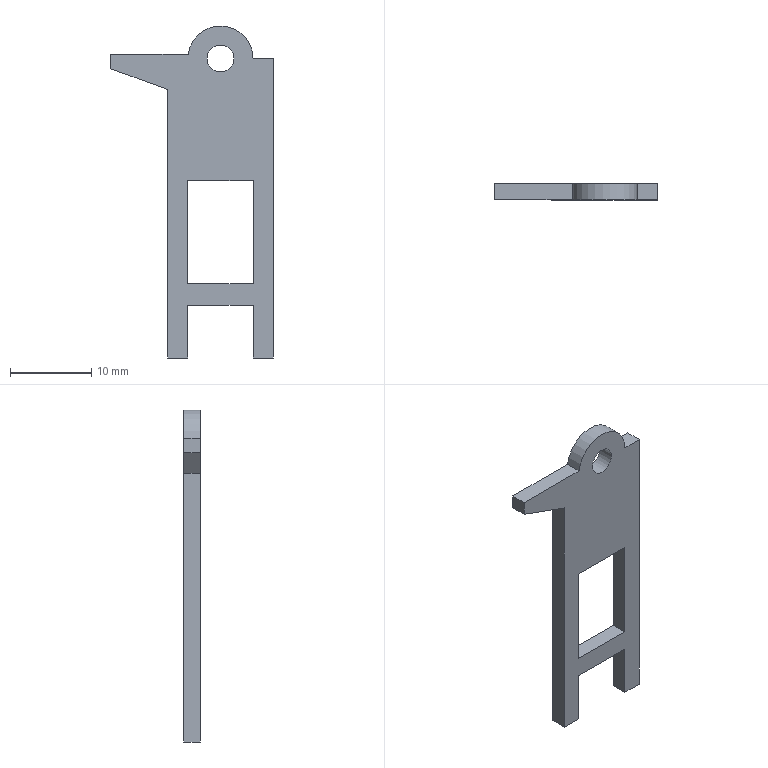Part | NX | 1 solid | 19 faces | box 20 x 2 x 40.8 mm | volume 727.635 mm3 | plane 17 | cylinder 2 | commonest cylinder face diameters 3.3 x1 8 x1
STEP:
#1=CARTESIAN_POINT('',(11.,81.5,41.85));
#2=VERTEX_POINT('',#1);
#3=CARTESIAN_POINT('',(11.,81.5,40.2));
#4=DIRECTION('',(0.,-1.,0.));
#5=DIRECTION('',(0.,0.,1.));
#6=AXIS2_PLACEMENT_3D('',#3,#4,#5);
#7=CIRCLE('',#6,1.65);
#8=EDGE_CURVE('',#2,#2,#7,.T.);
#9=ORIENTED_EDGE('',*,*,#8,.T.);
#10=EDGE_LOOP('',(#9));
#11=FACE_BOUND('',#10,.T.);
#12=CARTESIAN_POINT('',(4.5,81.5,3.4));
#13=VERTEX_POINT('',#12);
#14=CARTESIAN_POINT('',(7.,81.5,3.4));
#15=VERTEX_POINT('',#14);
#16=CARTESIAN_POINT('',(4.5,81.5,3.4));
#17=DIRECTION('',(1.,0.,0.));
#18=VECTOR('',#17,1000.);
#19=LINE('',#16,#18);
#20=EDGE_CURVE('',#13,#15,#19,.T.);
#21=ORIENTED_EDGE('',*,*,#20,.F.);
#22=CARTESIAN_POINT('',(4.5,81.5,36.4));
#23=VERTEX_POINT('',#22);
#24=CARTESIAN_POINT('',(4.5,81.5,3.4));
#25=DIRECTION('',(0.,0.,-1.));
#26=VECTOR('',#25,1000.);
#27=LINE('',#24,#26);
#28=EDGE_CURVE('',#23,#13,#27,.T.);
#29=ORIENTED_EDGE('',*,*,#28,.F.);
#30=CARTESIAN_POINT('',(-2.5,81.5,38.948));
#31=VERTEX_POINT('',#30);
#32=CARTESIAN_POINT('',(-2.5,81.5,38.948));
#33=DIRECTION('',(0.9397,0.,-0.342));
#34=VECTOR('',#33,1000.);
#35=LINE('',#32,#34);
#36=EDGE_CURVE('',#31,#23,#35,.T.);
#37=ORIENTED_EDGE('',*,*,#36,.F.);
#38=CARTESIAN_POINT('',(-2.5,81.5,40.7));
#39=VERTEX_POINT('',#38);
#40=CARTESIAN_POINT('',(-2.5,81.5,40.7));
#41=DIRECTION('',(0.,0.,-1.));
#42=VECTOR('',#41,1000.);
#43=LINE('',#40,#42);
#44=EDGE_CURVE('',#39,#31,#43,.T.);
#45=ORIENTED_EDGE('',*,*,#44,.F.);
#46=CARTESIAN_POINT('',(7.031,81.5,40.7));
#47=VERTEX_POINT('',#46);
#48=CARTESIAN_POINT('',(-2.5,81.5,40.7));
#49=DIRECTION('',(-1.,0.,0.));
#50=VECTOR('',#49,1000.);
#51=LINE('',#48,#50);
#52=EDGE_CURVE('',#47,#39,#51,.T.);
#53=ORIENTED_EDGE('',*,*,#52,.F.);
#54=CARTESIAN_POINT('',(15.,81.5,40.2));
#55=VERTEX_POINT('',#54);
#56=CARTESIAN_POINT('',(11.,81.5,40.2));
#57=DIRECTION('',(0.,-1.,0.));
#58=DIRECTION('',(0.,0.,-1.));
#59=AXIS2_PLACEMENT_3D('',#56,#57,#58);
#60=CIRCLE('',#59,4.);
#61=EDGE_CURVE('',#55,#47,#60,.T.);
#62=ORIENTED_EDGE('',*,*,#61,.F.);
#63=CARTESIAN_POINT('',(17.5,81.5,40.2));
#64=VERTEX_POINT('',#63);
#65=CARTESIAN_POINT('',(15.,81.5,40.2));
#66=DIRECTION('',(-1.,0.,0.));
#67=VECTOR('',#66,1000.);
#68=LINE('',#65,#67);
#69=EDGE_CURVE('',#64,#55,#68,.T.);
#70=ORIENTED_EDGE('',*,*,#69,.F.);
#71=CARTESIAN_POINT('',(17.5,81.5,3.4));
#72=VERTEX_POINT('',#71);
#73=CARTESIAN_POINT('',(17.5,81.5,3.4));
#74=DIRECTION('',(0.,0.,1.));
#75=VECTOR('',#74,1000.);
#76=LINE('',#73,#75);
#77=EDGE_CURVE('',#72,#64,#76,.T.);
#78=ORIENTED_EDGE('',*,*,#77,.F.);
#79=CARTESIAN_POINT('',(15.,81.5,3.4));
#80=VERTEX_POINT('',#79);
#81=CARTESIAN_POINT('',(15.,81.5,3.4));
#82=DIRECTION('',(1.,0.,0.));
#83=VECTOR('',#82,1000.);
#84=LINE('',#81,#83);
#85=EDGE_CURVE('',#80,#72,#84,.T.);
#86=ORIENTED_EDGE('',*,*,#85,.F.);
#87=CARTESIAN_POINT('',(15.,81.5,9.9));
#88=VERTEX_POINT('',#87);
#89=CARTESIAN_POINT('',(15.,81.5,3.4));
#90=DIRECTION('',(0.,0.,-1.));
#91=VECTOR('',#90,1000.);
#92=LINE('',#89,#91);
#93=EDGE_CURVE('',#88,#80,#92,.T.);
#94=ORIENTED_EDGE('',*,*,#93,.F.);
#95=CARTESIAN_POINT('',(7.,81.5,9.9));
#96=VERTEX_POINT('',#95);
#97=CARTESIAN_POINT('',(7.,81.5,9.9));
#98=DIRECTION('',(1.,0.,0.));
#99=VECTOR('',#98,1000.);
#100=LINE('',#97,#99);
#101=EDGE_CURVE('',#96,#88,#100,.T.);
#102=ORIENTED_EDGE('',*,*,#101,.F.);
#103=CARTESIAN_POINT('',(7.,81.5,3.4));
#104=DIRECTION('',(0.,0.,1.));
#105=VECTOR('',#104,1000.);
#106=LINE('',#103,#105);
#107=EDGE_CURVE('',#15,#96,#106,.T.);
#108=ORIENTED_EDGE('',*,*,#107,.F.);
#109=EDGE_LOOP('',(#21,#29,#37,#45,#53,#62,#70,#78,#86,#94,#102,#108));
#110=FACE_BOUND('',#109,.T.);
#111=CARTESIAN_POINT('',(7.,81.5,25.2));
#112=VERTEX_POINT('',#111);
#113=CARTESIAN_POINT('',(7.,81.5,12.5));
#114=VERTEX_POINT('',#113);
#115=CARTESIAN_POINT('',(7.,81.5,12.5));
#116=DIRECTION('',(0.,0.,-1.));
#117=VECTOR('',#116,1000.);
#118=LINE('',#115,#117);
#119=EDGE_CURVE('',#112,#114,#118,.T.);
#120=ORIENTED_EDGE('',*,*,#119,.T.);
#121=CARTESIAN_POINT('',(15.,81.5,12.5));
#122=VERTEX_POINT('',#121);
#123=CARTESIAN_POINT('',(7.,81.5,12.5));
#124=DIRECTION('',(1.,0.,0.));
#125=VECTOR('',#124,1000.);
#126=LINE('',#123,#125);
#127=EDGE_CURVE('',#114,#122,#126,.T.);
#128=ORIENTED_EDGE('',*,*,#127,.T.);
#129=CARTESIAN_POINT('',(15.,81.5,25.2));
#130=VERTEX_POINT('',#129);
#131=CARTESIAN_POINT('',(15.,81.5,12.5));
#132=DIRECTION('',(0.,0.,1.));
#133=VECTOR('',#132,1000.);
#134=LINE('',#131,#133);
#135=EDGE_CURVE('',#122,#130,#134,.T.);
#136=ORIENTED_EDGE('',*,*,#135,.T.);
#137=CARTESIAN_POINT('',(7.,81.5,25.2));
#138=DIRECTION('',(-1.,0.,0.));
#139=VECTOR('',#138,1000.);
#140=LINE('',#137,#139);
#141=EDGE_CURVE('',#130,#112,#140,.T.);
#142=ORIENTED_EDGE('',*,*,#141,.T.);
#143=EDGE_LOOP('',(#120,#128,#136,#142));
#144=FACE_BOUND('',#143,.T.);
#145=CARTESIAN_POINT('',(11.,81.5,40.2));
#146=DIRECTION('',(0.,1.,0.));
#147=DIRECTION('',(0.,0.,-1.));
#148=AXIS2_PLACEMENT_3D('',#145,#146,#147);
#149=PLANE('',#148);
#150=ADVANCED_FACE('',(#11,#110,#144),#149,.T.);
#151=CARTESIAN_POINT('',(11.,79.5,41.85));
#152=VERTEX_POINT('',#151);
#153=CARTESIAN_POINT('',(11.,79.5,40.2));
#154=DIRECTION('',(0.,-1.,0.));
#155=DIRECTION('',(0.,0.,1.));
#156=AXIS2_PLACEMENT_3D('',#153,#154,#155);
#157=CIRCLE('',#156,1.65);
#158=EDGE_CURVE('',#152,#152,#157,.T.);
#159=ORIENTED_EDGE('',*,*,#158,.F.);
#160=EDGE_LOOP('',(#159));
#161=FACE_BOUND('',#160,.T.);
#162=CARTESIAN_POINT('',(4.5,79.5,3.4));
#163=VERTEX_POINT('',#162);
#164=CARTESIAN_POINT('',(7.,79.5,3.4));
#165=VERTEX_POINT('',#164);
#166=CARTESIAN_POINT('',(4.5,79.5,3.4));
#167=DIRECTION('',(1.,0.,0.));
#168=VECTOR('',#167,1000.);
#169=LINE('',#166,#168);
#170=EDGE_CURVE('',#163,#165,#169,.T.);
#171=ORIENTED_EDGE('',*,*,#170,.T.);
#172=CARTESIAN_POINT('',(7.,79.5,9.9));
#173=VERTEX_POINT('',#172);
#174=CARTESIAN_POINT('',(7.,79.5,3.4));
#175=DIRECTION('',(0.,0.,1.));
#176=VECTOR('',#175,1000.);
#177=LINE('',#174,#176);
#178=EDGE_CURVE('',#165,#173,#177,.T.);
#179=ORIENTED_EDGE('',*,*,#178,.T.);
#180=CARTESIAN_POINT('',(15.,79.5,9.9));
#181=VERTEX_POINT('',#180);
#182=CARTESIAN_POINT('',(7.,79.5,9.9));
#183=DIRECTION('',(1.,0.,0.));
#184=VECTOR('',#183,1000.);
#185=LINE('',#182,#184);
#186=EDGE_CURVE('',#173,#181,#185,.T.);
#187=ORIENTED_EDGE('',*,*,#186,.T.);
#188=CARTESIAN_POINT('',(15.,79.5,3.4));
#189=VERTEX_POINT('',#188);
#190=CARTESIAN_POINT('',(15.,79.5,3.4));
#191=DIRECTION('',(0.,0.,-1.));
#192=VECTOR('',#191,1000.);
#193=LINE('',#190,#192);
#194=EDGE_CURVE('',#181,#189,#193,.T.);
#195=ORIENTED_EDGE('',*,*,#194,.T.);
#196=CARTESIAN_POINT('',(17.5,79.5,3.4));
#197=VERTEX_POINT('',#196);
#198=CARTESIAN_POINT('',(15.,79.5,3.4));
#199=DIRECTION('',(1.,0.,0.));
#200=VECTOR('',#199,1000.);
#201=LINE('',#198,#200);
#202=EDGE_CURVE('',#189,#197,#201,.T.);
#203=ORIENTED_EDGE('',*,*,#202,.T.);
#204=CARTESIAN_POINT('',(17.5,79.5,40.2));
#205=VERTEX_POINT('',#204);
#206=CARTESIAN_POINT('',(17.5,79.5,3.4));
#207=DIRECTION('',(0.,0.,1.));
#208=VECTOR('',#207,1000.);
#209=LINE('',#206,#208);
#210=EDGE_CURVE('',#197,#205,#209,.T.);
#211=ORIENTED_EDGE('',*,*,#210,.T.);
#212=CARTESIAN_POINT('',(15.,79.5,40.2));
#213=VERTEX_POINT('',#212);
#214=CARTESIAN_POINT('',(15.,79.5,40.2));
#215=DIRECTION('',(-1.,0.,0.));
#216=VECTOR('',#215,1000.);
#217=LINE('',#214,#216);
#218=EDGE_CURVE('',#205,#213,#217,.T.);
#219=ORIENTED_EDGE('',*,*,#218,.T.);
#220=CARTESIAN_POINT('',(7.031,79.5,40.7));
#221=VERTEX_POINT('',#220);
#222=CARTESIAN_POINT('',(11.,79.5,40.2));
#223=DIRECTION('',(0.,-1.,0.));
#224=DIRECTION('',(0.,0.,-1.));
#225=AXIS2_PLACEMENT_3D('',#222,#223,#224);
#226=CIRCLE('',#225,4.);
#227=EDGE_CURVE('',#213,#221,#226,.T.);
#228=ORIENTED_EDGE('',*,*,#227,.T.);
#229=CARTESIAN_POINT('',(-2.5,79.5,40.7));
#230=VERTEX_POINT('',#229);
#231=CARTESIAN_POINT('',(-2.5,79.5,40.7));
#232=DIRECTION('',(-1.,0.,0.));
#233=VECTOR('',#232,1000.);
#234=LINE('',#231,#233);
#235=EDGE_CURVE('',#221,#230,#234,.T.);
#236=ORIENTED_EDGE('',*,*,#235,.T.);
#237=CARTESIAN_POINT('',(-2.5,79.5,38.948));
#238=VERTEX_POINT('',#237);
#239=CARTESIAN_POINT('',(-2.5,79.5,40.7));
#240=DIRECTION('',(0.,0.,-1.));
#241=VECTOR('',#240,1000.);
#242=LINE('',#239,#241);
#243=EDGE_CURVE('',#230,#238,#242,.T.);
#244=ORIENTED_EDGE('',*,*,#243,.T.);
#245=CARTESIAN_POINT('',(4.5,79.5,36.4));
#246=VERTEX_POINT('',#245);
#247=CARTESIAN_POINT('',(-2.5,79.5,38.948));
#248=DIRECTION('',(0.9397,0.,-0.342));
#249=VECTOR('',#248,1000.);
#250=LINE('',#247,#249);
#251=EDGE_CURVE('',#238,#246,#250,.T.);
#252=ORIENTED_EDGE('',*,*,#251,.T.);
#253=CARTESIAN_POINT('',(4.5,79.5,3.4));
#254=DIRECTION('',(0.,0.,-1.));
#255=VECTOR('',#254,1000.);
#256=LINE('',#253,#255);
#257=EDGE_CURVE('',#246,#163,#256,.T.);
#258=ORIENTED_EDGE('',*,*,#257,.T.);
#259=EDGE_LOOP('',(#171,#179,#187,#195,#203,#211,#219,#228,#236,#244,#252,#258));
#260=FACE_BOUND('',#259,.T.);
#261=CARTESIAN_POINT('',(7.,79.5,12.5));
#262=VERTEX_POINT('',#261);
#263=CARTESIAN_POINT('',(15.,79.5,12.5));
#264=VERTEX_POINT('',#263);
#265=CARTESIAN_POINT('',(7.,79.5,12.5));
#266=DIRECTION('',(1.,0.,0.));
#267=VECTOR('',#266,1000.);
#268=LINE('',#265,#267);
#269=EDGE_CURVE('',#262,#264,#268,.T.);
#270=ORIENTED_EDGE('',*,*,#269,.F.);
#271=CARTESIAN_POINT('',(7.,79.5,25.2));
#272=VERTEX_POINT('',#271);
#273=CARTESIAN_POINT('',(7.,79.5,12.5));
#274=DIRECTION('',(0.,0.,-1.));
#275=VECTOR('',#274,1000.);
#276=LINE('',#273,#275);
#277=EDGE_CURVE('',#272,#262,#276,.T.);
#278=ORIENTED_EDGE('',*,*,#277,.F.);
#279=CARTESIAN_POINT('',(15.,79.5,25.2));
#280=VERTEX_POINT('',#279);
#281=CARTESIAN_POINT('',(7.,79.5,25.2));
#282=DIRECTION('',(-1.,0.,0.));
#283=VECTOR('',#282,1000.);
#284=LINE('',#281,#283);
#285=EDGE_CURVE('',#280,#272,#284,.T.);
#286=ORIENTED_EDGE('',*,*,#285,.F.);
#287=CARTESIAN_POINT('',(15.,79.5,12.5));
#288=DIRECTION('',(0.,0.,1.));
#289=VECTOR('',#288,1000.);
#290=LINE('',#287,#289);
#291=EDGE_CURVE('',#264,#280,#290,.T.);
#292=ORIENTED_EDGE('',*,*,#291,.F.);
#293=EDGE_LOOP('',(#270,#278,#286,#292));
#294=FACE_BOUND('',#293,.T.);
#295=CARTESIAN_POINT('',(11.,79.5,40.2));
#296=DIRECTION('',(0.,1.,0.));
#297=DIRECTION('',(0.,0.,-1.));
#298=AXIS2_PLACEMENT_3D('',#295,#296,#297);
#299=PLANE('',#298);
#300=ADVANCED_FACE('',(#161,#260,#294),#299,.F.);
#301=ORIENTED_EDGE('',*,*,#20,.T.);
#302=CARTESIAN_POINT('',(7.,79.5,3.4));
#303=DIRECTION('',(0.,1.,0.));
#304=VECTOR('',#303,1000.);
#305=LINE('',#302,#304);
#306=EDGE_CURVE('',#165,#15,#305,.T.);
#307=ORIENTED_EDGE('',*,*,#306,.F.);
#308=ORIENTED_EDGE('',*,*,#170,.F.);
#309=CARTESIAN_POINT('',(4.5,79.5,3.4));
#310=DIRECTION('',(0.,1.,0.));
#311=VECTOR('',#310,1000.);
#312=LINE('',#309,#311);
#313=EDGE_CURVE('',#163,#13,#312,.T.);
#314=ORIENTED_EDGE('',*,*,#313,.T.);
#315=EDGE_LOOP('',(#301,#307,#308,#314));
#316=FACE_BOUND('',#315,.T.);
#317=CARTESIAN_POINT('',(4.5,79.5,3.4));
#318=DIRECTION('',(0.,0.,1.));
#319=DIRECTION('',(0.,1.,0.));
#320=AXIS2_PLACEMENT_3D('',#317,#318,#319);
#321=PLANE('',#320);
#322=ADVANCED_FACE('',(#316),#321,.F.);
#323=ORIENTED_EDGE('',*,*,#107,.T.);
#324=CARTESIAN_POINT('',(7.,79.5,9.9));
#325=DIRECTION('',(0.,1.,0.));
#326=VECTOR('',#325,1000.);
#327=LINE('',#324,#326);
#328=EDGE_CURVE('',#173,#96,#327,.T.);
#329=ORIENTED_EDGE('',*,*,#328,.F.);
#330=ORIENTED_EDGE('',*,*,#178,.F.);
#331=ORIENTED_EDGE('',*,*,#306,.T.);
#332=EDGE_LOOP('',(#323,#329,#330,#331));
#333=FACE_BOUND('',#332,.T.);
#334=CARTESIAN_POINT('',(7.,79.5,3.4));
#335=DIRECTION('',(-1.,0.,0.));
#336=DIRECTION('',(0.,0.,-1.));
#337=AXIS2_PLACEMENT_3D('',#334,#335,#336);
#338=PLANE('',#337);
#339=ADVANCED_FACE('',(#333),#338,.F.);
#340=ORIENTED_EDGE('',*,*,#101,.T.);
#341=CARTESIAN_POINT('',(15.,79.5,9.9));
#342=DIRECTION('',(0.,1.,0.));
#343=VECTOR('',#342,1000.);
#344=LINE('',#341,#343);
#345=EDGE_CURVE('',#181,#88,#344,.T.);
#346=ORIENTED_EDGE('',*,*,#345,.F.);
#347=ORIENTED_EDGE('',*,*,#186,.F.);
#348=ORIENTED_EDGE('',*,*,#328,.T.);
#349=EDGE_LOOP('',(#340,#346,#347,#348));
#350=FACE_BOUND('',#349,.T.);
#351=CARTESIAN_POINT('',(7.,79.5,9.9));
#352=DIRECTION('',(0.,0.,1.));
#353=DIRECTION('',(0.,1.,0.));
#354=AXIS2_PLACEMENT_3D('',#351,#352,#353);
#355=PLANE('',#354);
#356=ADVANCED_FACE('',(#350),#355,.F.);
#357=ORIENTED_EDGE('',*,*,#93,.T.);
#358=CARTESIAN_POINT('',(15.,79.5,3.4));
#359=DIRECTION('',(0.,1.,0.));
#360=VECTOR('',#359,1000.);
#361=LINE('',#358,#360);
#362=EDGE_CURVE('',#189,#80,#361,.T.);
#363=ORIENTED_EDGE('',*,*,#362,.F.);
#364=ORIENTED_EDGE('',*,*,#194,.F.);
#365=ORIENTED_EDGE('',*,*,#345,.T.);
#366=EDGE_LOOP('',(#357,#363,#364,#365));
#367=FACE_BOUND('',#366,.T.);
#368=CARTESIAN_POINT('',(15.,79.5,3.4));
#369=DIRECTION('',(1.,0.,0.));
#370=DIRECTION('',(0.,0.,1.));
#371=AXIS2_PLACEMENT_3D('',#368,#369,#370);
#372=PLANE('',#371);
#373=ADVANCED_FACE('',(#367),#372,.F.);
#374=ORIENTED_EDGE('',*,*,#85,.T.);
#375=CARTESIAN_POINT('',(17.5,79.5,3.4));
#376=DIRECTION('',(0.,1.,0.));
#377=VECTOR('',#376,1000.);
#378=LINE('',#375,#377);
#379=EDGE_CURVE('',#197,#72,#378,.T.);
#380=ORIENTED_EDGE('',*,*,#379,.F.);
#381=ORIENTED_EDGE('',*,*,#202,.F.);
#382=ORIENTED_EDGE('',*,*,#362,.T.);
#383=EDGE_LOOP('',(#374,#380,#381,#382));
#384=FACE_BOUND('',#383,.T.);
#385=CARTESIAN_POINT('',(15.,79.5,3.4));
#386=DIRECTION('',(0.,0.,1.));
#387=DIRECTION('',(0.,1.,0.));
#388=AXIS2_PLACEMENT_3D('',#385,#386,#387);
#389=PLANE('',#388);
#390=ADVANCED_FACE('',(#384),#389,.F.);
#391=ORIENTED_EDGE('',*,*,#77,.T.);
#392=CARTESIAN_POINT('',(17.5,79.5,40.2));
#393=DIRECTION('',(0.,1.,0.));
#394=VECTOR('',#393,1000.);
#395=LINE('',#392,#394);
#396=EDGE_CURVE('',#205,#64,#395,.T.);
#397=ORIENTED_EDGE('',*,*,#396,.F.);
#398=ORIENTED_EDGE('',*,*,#210,.F.);
#399=ORIENTED_EDGE('',*,*,#379,.T.);
#400=EDGE_LOOP('',(#391,#397,#398,#399));
#401=FACE_BOUND('',#400,.T.);
#402=CARTESIAN_POINT('',(17.5,79.5,3.4));
#403=DIRECTION('',(-1.,0.,0.));
#404=DIRECTION('',(0.,0.,-1.));
#405=AXIS2_PLACEMENT_3D('',#402,#403,#404);
#406=PLANE('',#405);
#407=ADVANCED_FACE('',(#401),#406,.F.);
#408=ORIENTED_EDGE('',*,*,#69,.T.);
#409=CARTESIAN_POINT('',(15.,79.5,40.2));
#410=DIRECTION('',(0.,1.,0.));
#411=VECTOR('',#410,1000.);
#412=LINE('',#409,#411);
#413=EDGE_CURVE('',#213,#55,#412,.T.);
#414=ORIENTED_EDGE('',*,*,#413,.F.);
#415=ORIENTED_EDGE('',*,*,#218,.F.);
#416=ORIENTED_EDGE('',*,*,#396,.T.);
#417=EDGE_LOOP('',(#408,#414,#415,#416));
#418=FACE_BOUND('',#417,.T.);
#419=CARTESIAN_POINT('',(15.,79.5,40.2));
#420=DIRECTION('',(0.,0.,-1.));
#421=DIRECTION('',(1.,0.,0.));
#422=AXIS2_PLACEMENT_3D('',#419,#420,#421);
#423=PLANE('',#422);
#424=ADVANCED_FACE('',(#418),#423,.F.);
#425=ORIENTED_EDGE('',*,*,#61,.T.);
#426=CARTESIAN_POINT('',(7.031,79.5,40.7));
#427=DIRECTION('',(0.,1.,0.));
#428=VECTOR('',#427,1000.);
#429=LINE('',#426,#428);
#430=EDGE_CURVE('',#221,#47,#429,.T.);
#431=ORIENTED_EDGE('',*,*,#430,.F.);
#432=ORIENTED_EDGE('',*,*,#227,.F.);
#433=ORIENTED_EDGE('',*,*,#413,.T.);
#434=EDGE_LOOP('',(#425,#431,#432,#433));
#435=FACE_BOUND('',#434,.T.);
#436=CARTESIAN_POINT('',(11.,79.5,40.2));
#437=DIRECTION('',(0.,1.,0.));
#438=DIRECTION('',(0.,0.,-1.));
#439=AXIS2_PLACEMENT_3D('',#436,#437,#438);
#440=CYLINDRICAL_SURFACE('',#439,4.);
#441=ADVANCED_FACE('',(#435),#440,.T.);
#442=ORIENTED_EDGE('',*,*,#52,.T.);
#443=CARTESIAN_POINT('',(-2.5,79.5,40.7));
#444=DIRECTION('',(0.,1.,0.));
#445=VECTOR('',#444,1000.);
#446=LINE('',#443,#445);
#447=EDGE_CURVE('',#230,#39,#446,.T.);
#448=ORIENTED_EDGE('',*,*,#447,.F.);
#449=ORIENTED_EDGE('',*,*,#235,.F.);
#450=ORIENTED_EDGE('',*,*,#430,.T.);
#451=EDGE_LOOP('',(#442,#448,#449,#450));
#452=FACE_BOUND('',#451,.T.);
#453=CARTESIAN_POINT('',(-2.5,79.5,40.7));
#454=DIRECTION('',(0.,0.,-1.));
#455=DIRECTION('',(1.,0.,0.));
#456=AXIS2_PLACEMENT_3D('',#453,#454,#455);
#457=PLANE('',#456);
#458=ADVANCED_FACE('',(#452),#457,.F.);
#459=ORIENTED_EDGE('',*,*,#44,.T.);
#460=CARTESIAN_POINT('',(-2.5,79.5,38.948));
#461=DIRECTION('',(0.,1.,0.));
#462=VECTOR('',#461,1000.);
#463=LINE('',#460,#462);
#464=EDGE_CURVE('',#238,#31,#463,.T.);
#465=ORIENTED_EDGE('',*,*,#464,.F.);
#466=ORIENTED_EDGE('',*,*,#243,.F.);
#467=ORIENTED_EDGE('',*,*,#447,.T.);
#468=EDGE_LOOP('',(#459,#465,#466,#467));
#469=FACE_BOUND('',#468,.T.);
#470=CARTESIAN_POINT('',(-2.5,79.5,40.7));
#471=DIRECTION('',(1.,0.,0.));
#472=DIRECTION('',(0.,0.,1.));
#473=AXIS2_PLACEMENT_3D('',#470,#471,#472);
#474=PLANE('',#473);
#475=ADVANCED_FACE('',(#469),#474,.F.);
#476=ORIENTED_EDGE('',*,*,#36,.T.);
#477=CARTESIAN_POINT('',(4.5,79.5,36.4));
#478=DIRECTION('',(0.,1.,0.));
#479=VECTOR('',#478,1000.);
#480=LINE('',#477,#479);
#481=EDGE_CURVE('',#246,#23,#480,.T.);
#482=ORIENTED_EDGE('',*,*,#481,.F.);
#483=ORIENTED_EDGE('',*,*,#251,.F.);
#484=ORIENTED_EDGE('',*,*,#464,.T.);
#485=EDGE_LOOP('',(#476,#482,#483,#484));
#486=FACE_BOUND('',#485,.T.);
#487=CARTESIAN_POINT('',(-2.5,79.5,38.948));
#488=DIRECTION('',(0.342,0.,0.9397));
#489=DIRECTION('',(-0.9397,0.,0.342));
#490=AXIS2_PLACEMENT_3D('',#487,#488,#489);
#491=PLANE('',#490);
#492=ADVANCED_FACE('',(#486),#491,.F.);
#493=ORIENTED_EDGE('',*,*,#28,.T.);
#494=ORIENTED_EDGE('',*,*,#313,.F.);
#495=ORIENTED_EDGE('',*,*,#257,.F.);
#496=ORIENTED_EDGE('',*,*,#481,.T.);
#497=EDGE_LOOP('',(#493,#494,#495,#496));
#498=FACE_BOUND('',#497,.T.);
#499=CARTESIAN_POINT('',(4.5,79.5,3.4));
#500=DIRECTION('',(1.,0.,0.));
#501=DIRECTION('',(0.,0.,1.));
#502=AXIS2_PLACEMENT_3D('',#499,#500,#501);
#503=PLANE('',#502);
#504=ADVANCED_FACE('',(#498),#503,.F.);
#505=ORIENTED_EDGE('',*,*,#158,.T.);
#506=EDGE_LOOP('',(#505));
#507=FACE_BOUND('',#506,.T.);
#508=ORIENTED_EDGE('',*,*,#8,.F.);
#509=EDGE_LOOP('',(#508));
#510=FACE_BOUND('',#509,.T.);
#511=CARTESIAN_POINT('',(11.,79.5,40.2));
#512=DIRECTION('',(0.,1.,0.));
#513=DIRECTION('',(0.,0.,-1.));
#514=AXIS2_PLACEMENT_3D('',#511,#512,#513);
#515=CYLINDRICAL_SURFACE('',#514,1.65);
#516=ADVANCED_FACE('',(#507,#510),#515,.F.);
#517=ORIENTED_EDGE('',*,*,#127,.F.);
#518=CARTESIAN_POINT('',(7.,79.5,12.5));
#519=DIRECTION('',(0.,1.,0.));
#520=VECTOR('',#519,1000.);
#521=LINE('',#518,#520);
#522=EDGE_CURVE('',#262,#114,#521,.T.);
#523=ORIENTED_EDGE('',*,*,#522,.F.);
#524=ORIENTED_EDGE('',*,*,#269,.T.);
#525=CARTESIAN_POINT('',(15.,79.5,12.5));
#526=DIRECTION('',(0.,1.,0.));
#527=VECTOR('',#526,1000.);
#528=LINE('',#525,#527);
#529=EDGE_CURVE('',#264,#122,#528,.T.);
#530=ORIENTED_EDGE('',*,*,#529,.T.);
#531=EDGE_LOOP('',(#517,#523,#524,#530));
#532=FACE_BOUND('',#531,.T.);
#533=CARTESIAN_POINT('',(7.,79.5,12.5));
#534=DIRECTION('',(0.,0.,1.));
#535=DIRECTION('',(0.,1.,0.));
#536=AXIS2_PLACEMENT_3D('',#533,#534,#535);
#537=PLANE('',#536);
#538=ADVANCED_FACE('',(#532),#537,.T.);
#539=ORIENTED_EDGE('',*,*,#135,.F.);
#540=ORIENTED_EDGE('',*,*,#529,.F.);
#541=ORIENTED_EDGE('',*,*,#291,.T.);
#542=CARTESIAN_POINT('',(15.,79.5,25.2));
#543=DIRECTION('',(0.,1.,0.));
#544=VECTOR('',#543,1000.);
#545=LINE('',#542,#544);
#546=EDGE_CURVE('',#280,#130,#545,.T.);
#547=ORIENTED_EDGE('',*,*,#546,.T.);
#548=EDGE_LOOP('',(#539,#540,#541,#547));
#549=FACE_BOUND('',#548,.T.);
#550=CARTESIAN_POINT('',(15.,79.5,12.5));
#551=DIRECTION('',(-1.,0.,0.));
#552=DIRECTION('',(0.,0.,-1.));
#553=AXIS2_PLACEMENT_3D('',#550,#551,#552);
#554=PLANE('',#553);
#555=ADVANCED_FACE('',(#549),#554,.T.);
#556=ORIENTED_EDGE('',*,*,#141,.F.);
#557=ORIENTED_EDGE('',*,*,#546,.F.);
#558=ORIENTED_EDGE('',*,*,#285,.T.);
#559=CARTESIAN_POINT('',(7.,79.5,25.2));
#560=DIRECTION('',(0.,1.,0.));
#561=VECTOR('',#560,1000.);
#562=LINE('',#559,#561);
#563=EDGE_CURVE('',#272,#112,#562,.T.);
#564=ORIENTED_EDGE('',*,*,#563,.T.);
#565=EDGE_LOOP('',(#556,#557,#558,#564));
#566=FACE_BOUND('',#565,.T.);
#567=CARTESIAN_POINT('',(7.,79.5,25.2));
#568=DIRECTION('',(0.,0.,-1.));
#569=DIRECTION('',(1.,0.,0.));
#570=AXIS2_PLACEMENT_3D('',#567,#568,#569);
#571=PLANE('',#570);
#572=ADVANCED_FACE('',(#566),#571,.T.);
#573=ORIENTED_EDGE('',*,*,#119,.F.);
#574=ORIENTED_EDGE('',*,*,#563,.F.);
#575=ORIENTED_EDGE('',*,*,#277,.T.);
#576=ORIENTED_EDGE('',*,*,#522,.T.);
#577=EDGE_LOOP('',(#573,#574,#575,#576));
#578=FACE_BOUND('',#577,.T.);
#579=CARTESIAN_POINT('',(7.,79.5,12.5));
#580=DIRECTION('',(1.,0.,0.));
#581=DIRECTION('',(0.,0.,1.));
#582=AXIS2_PLACEMENT_3D('',#579,#580,#581);
#583=PLANE('',#582);
#584=ADVANCED_FACE('',(#578),#583,.T.);
#585=CLOSED_SHELL('',(#150,#300,#322,#339,#356,#373,#390,#407,#424,#441,#458,#475,#492,#504,#516,#538,#555,#572,#584));
#586=MANIFOLD_SOLID_BREP('',#585);
#587=(LENGTH_UNIT()NAMED_UNIT(*)SI_UNIT(.MILLI.,.METRE.));
#588=UNCERTAINTY_MEASURE_WITH_UNIT(LENGTH_MEASURE(0.00001),#587,'','');
#589=(NAMED_UNIT(*)PLANE_ANGLE_UNIT()SI_UNIT($,.RADIAN.));
#590=(NAMED_UNIT(*)SI_UNIT($,.STERADIAN.)SOLID_ANGLE_UNIT());
#591=(GEOMETRIC_REPRESENTATION_CONTEXT(3)GLOBAL_UNCERTAINTY_ASSIGNED_CONTEXT((#588))GLOBAL_UNIT_ASSIGNED_CONTEXT((#587,#589,#590))REPRESENTATION_CONTEXT('',''));
#592=ADVANCED_BREP_SHAPE_REPRESENTATION('',(#586),#591);